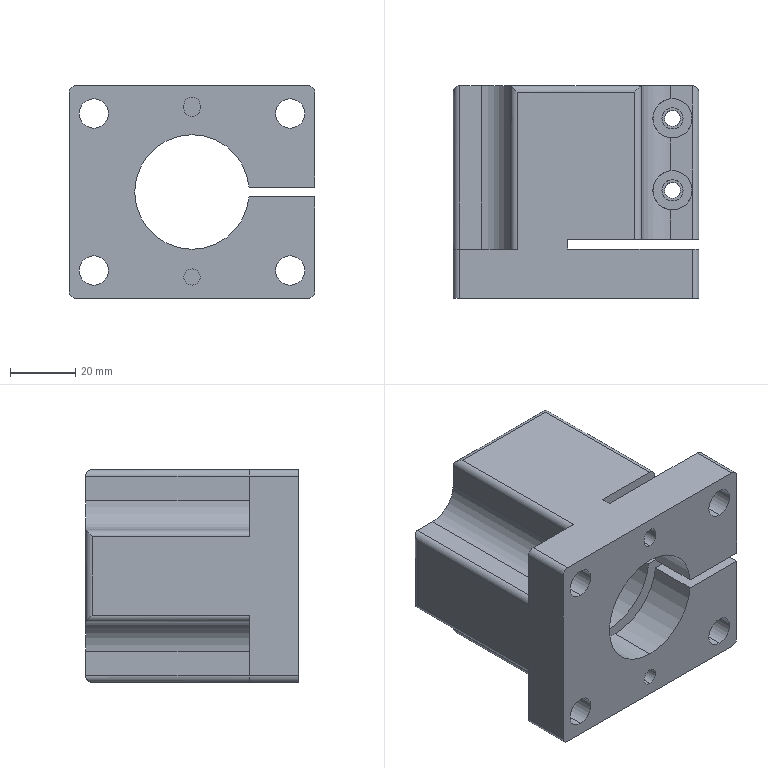Part | SolidWorks | features BaseBody 1 | 1 solid | 88 faces | box 75 x 65 x 65 mm | volume 177791 mm3 | cylinder 51 | plane 37 | commonest cylinder face diameters 4 x17 9 x8 5 x5 35 x5 4.917 x4 6.5 x4